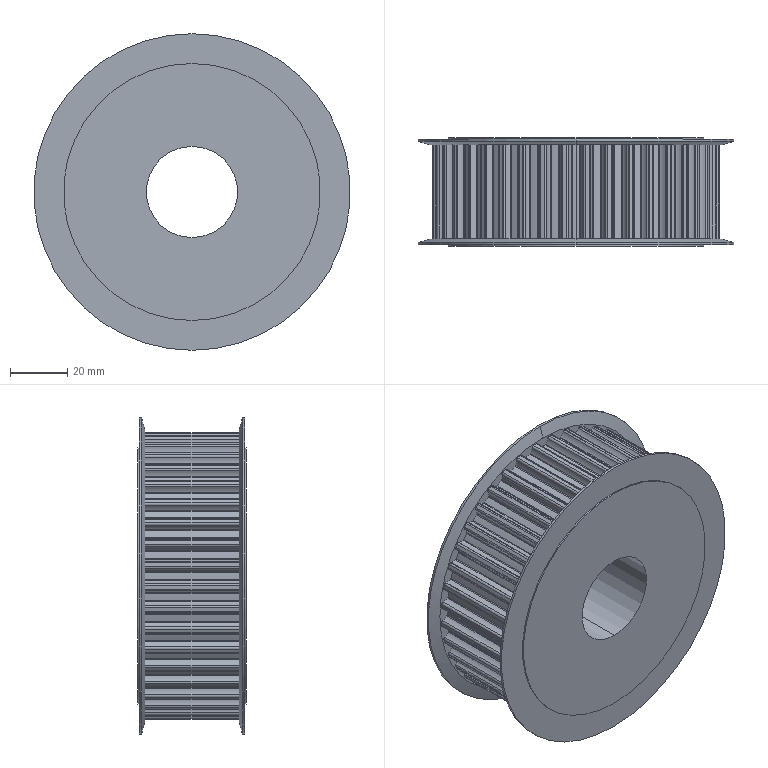Part | SolidWorks | features BaseBody 1 | 1 solid | 377 faces | box 110.9 x 38 x 110.9 mm | volume 257710 mm3 | cylinder 367 | plane 6 | cone 4 | commonest cylinder face diameters 1.5 x98 0.8 x92 10.6 x86 94.83 x41 100.49 x40 90 x4